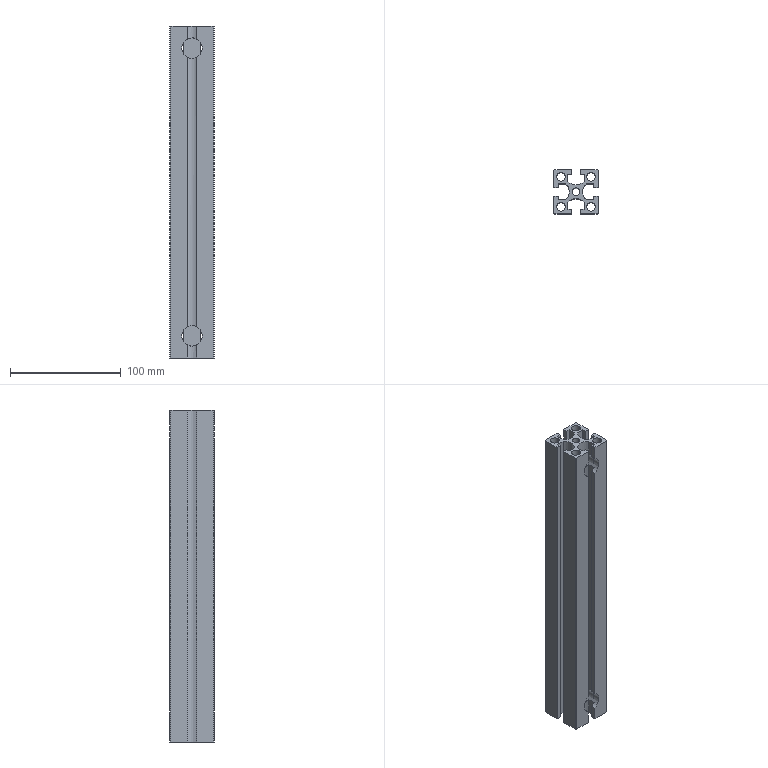Part | STEP file | 09-06 aluminium profile 4040-500 | 1 solid | 93 faces | box 40 x 40 x 300 mm | volume 207088 mm3 | plane 62 | cylinder 31 | commonest cylinder face diameters 19 x9 8 x8 18.5 x8 2 x4 6.8 x2